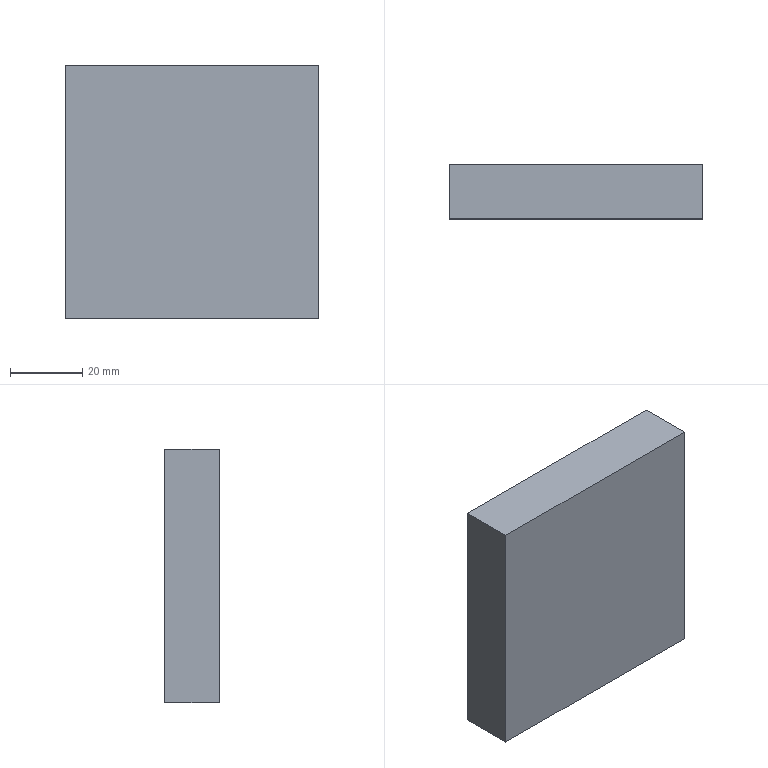Part | STEP file | Tube feed_id682_x_t | 1 solid | 6 faces | box 70 x 15 x 70 mm | volume 73500 mm3 | plane 6
STEP:
#1=CARTESIAN_POINT('',(0.,0.,0.));
#2=DIRECTION('',(0.,0.,1.));
#3=DIRECTION('',(1.,0.,0.));
#4=AXIS2_PLACEMENT_3D('',#1,#2,#3);
#5=CARTESIAN_POINT('',(141.,175.936,-50.15));
#6=VERTEX_POINT('',#5);
#7=CARTESIAN_POINT('',(141.,160.936,-50.15));
#8=VERTEX_POINT('',#7);
#9=CARTESIAN_POINT('',(141.,175.936,-50.15));
#10=DIRECTION('',(0.,-1.,0.));
#11=VECTOR('',#10,1.);
#12=LINE('',#9,#11);
#13=CARTESIAN_POINT('',(141.,175.936,19.85));
#14=DIRECTION('',(1.,0.,0.));
#15=DIRECTION('',(0.,0.,-1.));
#16=AXIS2_PLACEMENT_3D('',#13,#14,#15);
#17=PLANE('',#16);
#18=CARTESIAN_POINT('',(70.,0.));
#19=DIRECTION('',(0.,-1.));
#20=VECTOR('',#19,1.);
#21=LINE('',#18,#20);
#22=(GEOMETRIC_REPRESENTATION_CONTEXT(2)PARAMETRIC_REPRESENTATION_CONTEXT()REPRESENTATION_CONTEXT('',''));
#23=DEFINITIONAL_REPRESENTATION('',(#21),#22);
#24=PCURVE('',#17,#23);
#25=CARTESIAN_POINT('',(0.,0.,-50.15));
#26=DIRECTION('',(0.,0.,1.));
#27=DIRECTION('',(1.,0.,0.));
#28=AXIS2_PLACEMENT_3D('',#25,#26,#27);
#29=PLANE('',#28);
#30=CARTESIAN_POINT('',(141.,175.936));
#31=DIRECTION('',(0.,-1.));
#32=VECTOR('',#31,1.);
#33=LINE('',#30,#32);
#34=(GEOMETRIC_REPRESENTATION_CONTEXT(2)PARAMETRIC_REPRESENTATION_CONTEXT()REPRESENTATION_CONTEXT('',''));
#35=DEFINITIONAL_REPRESENTATION('',(#33),#34);
#36=PCURVE('',#29,#35);
#37=SURFACE_CURVE('',#12,(#24,#36),.PCURVE_S1.);
#38=EDGE_CURVE('',#6,#8,#37,.T.);
#39=ORIENTED_EDGE('',*,*,#38,.T.);
#40=CARTESIAN_POINT('',(141.,160.936,19.85));
#41=VERTEX_POINT('',#40);
#42=CARTESIAN_POINT('',(141.,160.936,19.85));
#43=DIRECTION('',(0.,0.,-1.));
#44=VECTOR('',#43,1.);
#45=LINE('',#42,#44);
#46=CARTESIAN_POINT('',(0.,-15.));
#47=DIRECTION('',(1.,0.));
#48=VECTOR('',#47,1.);
#49=LINE('',#46,#48);
#50=(GEOMETRIC_REPRESENTATION_CONTEXT(2)PARAMETRIC_REPRESENTATION_CONTEXT()REPRESENTATION_CONTEXT('',''));
#51=DEFINITIONAL_REPRESENTATION('',(#49),#50);
#52=PCURVE('',#17,#51);
#53=CARTESIAN_POINT('',(141.,160.936,19.85));
#54=DIRECTION('',(0.,1.,0.));
#55=DIRECTION('',(-1.,0.,0.));
#56=AXIS2_PLACEMENT_3D('',#53,#54,#55);
#57=PLANE('',#56);
#58=CARTESIAN_POINT('',(0.,0.));
#59=DIRECTION('',(0.,-1.));
#60=VECTOR('',#59,1.);
#61=LINE('',#58,#60);
#62=(GEOMETRIC_REPRESENTATION_CONTEXT(2)PARAMETRIC_REPRESENTATION_CONTEXT()REPRESENTATION_CONTEXT('',''));
#63=DEFINITIONAL_REPRESENTATION('',(#61),#62);
#64=PCURVE('',#57,#63);
#65=SURFACE_CURVE('',#45,(#52,#64),.PCURVE_S1.);
#66=EDGE_CURVE('',#41,#8,#65,.T.);
#67=ORIENTED_EDGE('',*,*,#66,.F.);
#68=CARTESIAN_POINT('',(141.,175.936,19.85));
#69=VERTEX_POINT('',#68);
#70=CARTESIAN_POINT('',(141.,175.936,19.85));
#71=DIRECTION('',(0.,-1.,0.));
#72=VECTOR('',#71,1.);
#73=LINE('',#70,#72);
#74=CARTESIAN_POINT('',(0.,0.));
#75=DIRECTION('',(0.,-1.));
#76=VECTOR('',#75,1.);
#77=LINE('',#74,#76);
#78=(GEOMETRIC_REPRESENTATION_CONTEXT(2)PARAMETRIC_REPRESENTATION_CONTEXT()REPRESENTATION_CONTEXT('',''));
#79=DEFINITIONAL_REPRESENTATION('',(#77),#78);
#80=PCURVE('',#17,#79);
#81=CARTESIAN_POINT('',(0.,0.,19.85));
#82=DIRECTION('',(0.,0.,1.));
#83=DIRECTION('',(1.,0.,0.));
#84=AXIS2_PLACEMENT_3D('',#81,#82,#83);
#85=PLANE('',#84);
#86=CARTESIAN_POINT('',(141.,175.936));
#87=DIRECTION('',(0.,-1.));
#88=VECTOR('',#87,1.);
#89=LINE('',#86,#88);
#90=(GEOMETRIC_REPRESENTATION_CONTEXT(2)PARAMETRIC_REPRESENTATION_CONTEXT()REPRESENTATION_CONTEXT('',''));
#91=DEFINITIONAL_REPRESENTATION('',(#89),#90);
#92=PCURVE('',#85,#91);
#93=SURFACE_CURVE('',#73,(#80,#92),.PCURVE_S1.);
#94=EDGE_CURVE('',#69,#41,#93,.T.);
#95=ORIENTED_EDGE('',*,*,#94,.F.);
#96=CARTESIAN_POINT('',(141.,175.936,19.85));
#97=DIRECTION('',(0.,0.,-1.));
#98=VECTOR('',#97,1.);
#99=LINE('',#96,#98);
#100=CARTESIAN_POINT('',(0.,0.));
#101=DIRECTION('',(1.,0.));
#102=VECTOR('',#101,1.);
#103=LINE('',#100,#102);
#104=(GEOMETRIC_REPRESENTATION_CONTEXT(2)PARAMETRIC_REPRESENTATION_CONTEXT()REPRESENTATION_CONTEXT('',''));
#105=DEFINITIONAL_REPRESENTATION('',(#103),#104);
#106=PCURVE('',#17,#105);
#107=CARTESIAN_POINT('',(211.,175.936,19.85));
#108=DIRECTION('',(0.,-1.,0.));
#109=DIRECTION('',(0.,0.,-1.));
#110=AXIS2_PLACEMENT_3D('',#107,#108,#109);
#111=PLANE('',#110);
#112=CARTESIAN_POINT('',(0.,-70.));
#113=DIRECTION('',(1.,0.));
#114=VECTOR('',#113,1.);
#115=LINE('',#112,#114);
#116=(GEOMETRIC_REPRESENTATION_CONTEXT(2)PARAMETRIC_REPRESENTATION_CONTEXT()REPRESENTATION_CONTEXT('',''));
#117=DEFINITIONAL_REPRESENTATION('',(#115),#116);
#118=PCURVE('',#111,#117);
#119=SURFACE_CURVE('',#99,(#106,#118),.PCURVE_S1.);
#120=EDGE_CURVE('',#69,#6,#119,.T.);
#121=ORIENTED_EDGE('',*,*,#120,.T.);
#122=EDGE_LOOP('',(#39,#67,#95,#121));
#123=FACE_BOUND('',#122,.T.);
#124=ADVANCED_FACE('',(#123),#17,.F.);
#125=CARTESIAN_POINT('',(211.,160.936,-50.15));
#126=VERTEX_POINT('',#125);
#127=CARTESIAN_POINT('',(141.,160.936,-50.15));
#128=DIRECTION('',(1.,0.,0.));
#129=VECTOR('',#128,1.);
#130=LINE('',#127,#129);
#131=CARTESIAN_POINT('',(0.,-70.));
#132=DIRECTION('',(-1.,0.));
#133=VECTOR('',#132,1.);
#134=LINE('',#131,#133);
#135=(GEOMETRIC_REPRESENTATION_CONTEXT(2)PARAMETRIC_REPRESENTATION_CONTEXT()REPRESENTATION_CONTEXT('',''));
#136=DEFINITIONAL_REPRESENTATION('',(#134),#135);
#137=PCURVE('',#57,#136);
#138=CARTESIAN_POINT('',(141.,160.936));
#139=DIRECTION('',(1.,0.));
#140=VECTOR('',#139,1.);
#141=LINE('',#138,#140);
#142=(GEOMETRIC_REPRESENTATION_CONTEXT(2)PARAMETRIC_REPRESENTATION_CONTEXT()REPRESENTATION_CONTEXT('',''));
#143=DEFINITIONAL_REPRESENTATION('',(#141),#142);
#144=PCURVE('',#29,#143);
#145=SURFACE_CURVE('',#130,(#137,#144),.PCURVE_S1.);
#146=EDGE_CURVE('',#8,#126,#145,.T.);
#147=ORIENTED_EDGE('',*,*,#146,.T.);
#148=CARTESIAN_POINT('',(211.,160.936,19.85));
#149=VERTEX_POINT('',#148);
#150=CARTESIAN_POINT('',(211.,160.936,19.85));
#151=DIRECTION('',(0.,0.,-1.));
#152=VECTOR('',#151,1.);
#153=LINE('',#150,#152);
#154=CARTESIAN_POINT('',(-70.,0.));
#155=DIRECTION('',(0.,-1.));
#156=VECTOR('',#155,1.);
#157=LINE('',#154,#156);
#158=(GEOMETRIC_REPRESENTATION_CONTEXT(2)PARAMETRIC_REPRESENTATION_CONTEXT()REPRESENTATION_CONTEXT('',''));
#159=DEFINITIONAL_REPRESENTATION('',(#157),#158);
#160=PCURVE('',#57,#159);
#161=CARTESIAN_POINT('',(211.,160.936,19.85));
#162=DIRECTION('',(-1.,0.,0.));
#163=DIRECTION('',(0.,0.,1.));
#164=AXIS2_PLACEMENT_3D('',#161,#162,#163);
#165=PLANE('',#164);
#166=CARTESIAN_POINT('',(0.,0.));
#167=DIRECTION('',(-1.,0.));
#168=VECTOR('',#167,1.);
#169=LINE('',#166,#168);
#170=(GEOMETRIC_REPRESENTATION_CONTEXT(2)PARAMETRIC_REPRESENTATION_CONTEXT()REPRESENTATION_CONTEXT('',''));
#171=DEFINITIONAL_REPRESENTATION('',(#169),#170);
#172=PCURVE('',#165,#171);
#173=SURFACE_CURVE('',#153,(#160,#172),.PCURVE_S1.);
#174=EDGE_CURVE('',#149,#126,#173,.T.);
#175=ORIENTED_EDGE('',*,*,#174,.F.);
#176=CARTESIAN_POINT('',(141.,160.936,19.85));
#177=DIRECTION('',(1.,0.,0.));
#178=VECTOR('',#177,1.);
#179=LINE('',#176,#178);
#180=CARTESIAN_POINT('',(0.,0.));
#181=DIRECTION('',(-1.,0.));
#182=VECTOR('',#181,1.);
#183=LINE('',#180,#182);
#184=(GEOMETRIC_REPRESENTATION_CONTEXT(2)PARAMETRIC_REPRESENTATION_CONTEXT()REPRESENTATION_CONTEXT('',''));
#185=DEFINITIONAL_REPRESENTATION('',(#183),#184);
#186=PCURVE('',#57,#185);
#187=CARTESIAN_POINT('',(141.,160.936));
#188=DIRECTION('',(1.,0.));
#189=VECTOR('',#188,1.);
#190=LINE('',#187,#189);
#191=(GEOMETRIC_REPRESENTATION_CONTEXT(2)PARAMETRIC_REPRESENTATION_CONTEXT()REPRESENTATION_CONTEXT('',''));
#192=DEFINITIONAL_REPRESENTATION('',(#190),#191);
#193=PCURVE('',#85,#192);
#194=SURFACE_CURVE('',#179,(#186,#193),.PCURVE_S1.);
#195=EDGE_CURVE('',#41,#149,#194,.T.);
#196=ORIENTED_EDGE('',*,*,#195,.F.);
#197=ORIENTED_EDGE('',*,*,#66,.T.);
#198=EDGE_LOOP('',(#147,#175,#196,#197));
#199=FACE_BOUND('',#198,.T.);
#200=ADVANCED_FACE('',(#199),#57,.F.);
#201=CARTESIAN_POINT('',(211.,175.936,-50.15));
#202=VERTEX_POINT('',#201);
#203=CARTESIAN_POINT('',(211.,160.936,-50.15));
#204=DIRECTION('',(0.,1.,0.));
#205=VECTOR('',#204,1.);
#206=LINE('',#203,#205);
#207=CARTESIAN_POINT('',(-70.,0.));
#208=DIRECTION('',(0.,1.));
#209=VECTOR('',#208,1.);
#210=LINE('',#207,#209);
#211=(GEOMETRIC_REPRESENTATION_CONTEXT(2)PARAMETRIC_REPRESENTATION_CONTEXT()REPRESENTATION_CONTEXT('',''));
#212=DEFINITIONAL_REPRESENTATION('',(#210),#211);
#213=PCURVE('',#165,#212);
#214=CARTESIAN_POINT('',(211.,160.936));
#215=DIRECTION('',(0.,1.));
#216=VECTOR('',#215,1.);
#217=LINE('',#214,#216);
#218=(GEOMETRIC_REPRESENTATION_CONTEXT(2)PARAMETRIC_REPRESENTATION_CONTEXT()REPRESENTATION_CONTEXT('',''));
#219=DEFINITIONAL_REPRESENTATION('',(#217),#218);
#220=PCURVE('',#29,#219);
#221=SURFACE_CURVE('',#206,(#213,#220),.PCURVE_S1.);
#222=EDGE_CURVE('',#126,#202,#221,.T.);
#223=ORIENTED_EDGE('',*,*,#222,.T.);
#224=CARTESIAN_POINT('',(211.,175.936,19.85));
#225=VERTEX_POINT('',#224);
#226=CARTESIAN_POINT('',(211.,175.936,19.85));
#227=DIRECTION('',(0.,0.,-1.));
#228=VECTOR('',#227,1.);
#229=LINE('',#226,#228);
#230=CARTESIAN_POINT('',(0.,15.));
#231=DIRECTION('',(-1.,0.));
#232=VECTOR('',#231,1.);
#233=LINE('',#230,#232);
#234=(GEOMETRIC_REPRESENTATION_CONTEXT(2)PARAMETRIC_REPRESENTATION_CONTEXT()REPRESENTATION_CONTEXT('',''));
#235=DEFINITIONAL_REPRESENTATION('',(#233),#234);
#236=PCURVE('',#165,#235);
#237=CARTESIAN_POINT('',(0.,0.));
#238=DIRECTION('',(1.,0.));
#239=VECTOR('',#238,1.);
#240=LINE('',#237,#239);
#241=(GEOMETRIC_REPRESENTATION_CONTEXT(2)PARAMETRIC_REPRESENTATION_CONTEXT()REPRESENTATION_CONTEXT('',''));
#242=DEFINITIONAL_REPRESENTATION('',(#240),#241);
#243=PCURVE('',#111,#242);
#244=SURFACE_CURVE('',#229,(#236,#243),.PCURVE_S1.);
#245=EDGE_CURVE('',#225,#202,#244,.T.);
#246=ORIENTED_EDGE('',*,*,#245,.F.);
#247=CARTESIAN_POINT('',(211.,160.936,19.85));
#248=DIRECTION('',(0.,1.,0.));
#249=VECTOR('',#248,1.);
#250=LINE('',#247,#249);
#251=CARTESIAN_POINT('',(0.,0.));
#252=DIRECTION('',(0.,1.));
#253=VECTOR('',#252,1.);
#254=LINE('',#251,#253);
#255=(GEOMETRIC_REPRESENTATION_CONTEXT(2)PARAMETRIC_REPRESENTATION_CONTEXT()REPRESENTATION_CONTEXT('',''));
#256=DEFINITIONAL_REPRESENTATION('',(#254),#255);
#257=PCURVE('',#165,#256);
#258=CARTESIAN_POINT('',(211.,160.936));
#259=DIRECTION('',(0.,1.));
#260=VECTOR('',#259,1.);
#261=LINE('',#258,#260);
#262=(GEOMETRIC_REPRESENTATION_CONTEXT(2)PARAMETRIC_REPRESENTATION_CONTEXT()REPRESENTATION_CONTEXT('',''));
#263=DEFINITIONAL_REPRESENTATION('',(#261),#262);
#264=PCURVE('',#85,#263);
#265=SURFACE_CURVE('',#250,(#257,#264),.PCURVE_S1.);
#266=EDGE_CURVE('',#149,#225,#265,.T.);
#267=ORIENTED_EDGE('',*,*,#266,.F.);
#268=ORIENTED_EDGE('',*,*,#174,.T.);
#269=EDGE_LOOP('',(#223,#246,#267,#268));
#270=FACE_BOUND('',#269,.T.);
#271=ADVANCED_FACE('',(#270),#165,.F.);
#272=CARTESIAN_POINT('',(211.,175.936,-50.15));
#273=DIRECTION('',(-1.,0.,0.));
#274=VECTOR('',#273,1.);
#275=LINE('',#272,#274);
#276=CARTESIAN_POINT('',(70.,0.));
#277=DIRECTION('',(0.,-1.));
#278=VECTOR('',#277,1.);
#279=LINE('',#276,#278);
#280=(GEOMETRIC_REPRESENTATION_CONTEXT(2)PARAMETRIC_REPRESENTATION_CONTEXT()REPRESENTATION_CONTEXT('',''));
#281=DEFINITIONAL_REPRESENTATION('',(#279),#280);
#282=PCURVE('',#111,#281);
#283=CARTESIAN_POINT('',(211.,175.936));
#284=DIRECTION('',(-1.,0.));
#285=VECTOR('',#284,1.);
#286=LINE('',#283,#285);
#287=(GEOMETRIC_REPRESENTATION_CONTEXT(2)PARAMETRIC_REPRESENTATION_CONTEXT()REPRESENTATION_CONTEXT('',''));
#288=DEFINITIONAL_REPRESENTATION('',(#286),#287);
#289=PCURVE('',#29,#288);
#290=SURFACE_CURVE('',#275,(#282,#289),.PCURVE_S1.);
#291=EDGE_CURVE('',#202,#6,#290,.T.);
#292=ORIENTED_EDGE('',*,*,#291,.T.);
#293=ORIENTED_EDGE('',*,*,#120,.F.);
#294=CARTESIAN_POINT('',(211.,175.936,19.85));
#295=DIRECTION('',(-1.,0.,0.));
#296=VECTOR('',#295,1.);
#297=LINE('',#294,#296);
#298=CARTESIAN_POINT('',(0.,0.));
#299=DIRECTION('',(0.,-1.));
#300=VECTOR('',#299,1.);
#301=LINE('',#298,#300);
#302=(GEOMETRIC_REPRESENTATION_CONTEXT(2)PARAMETRIC_REPRESENTATION_CONTEXT()REPRESENTATION_CONTEXT('',''));
#303=DEFINITIONAL_REPRESENTATION('',(#301),#302);
#304=PCURVE('',#111,#303);
#305=CARTESIAN_POINT('',(211.,175.936));
#306=DIRECTION('',(-1.,0.));
#307=VECTOR('',#306,1.);
#308=LINE('',#305,#307);
#309=(GEOMETRIC_REPRESENTATION_CONTEXT(2)PARAMETRIC_REPRESENTATION_CONTEXT()REPRESENTATION_CONTEXT('',''));
#310=DEFINITIONAL_REPRESENTATION('',(#308),#309);
#311=PCURVE('',#85,#310);
#312=SURFACE_CURVE('',#297,(#304,#311),.PCURVE_S1.);
#313=EDGE_CURVE('',#225,#69,#312,.T.);
#314=ORIENTED_EDGE('',*,*,#313,.F.);
#315=ORIENTED_EDGE('',*,*,#245,.T.);
#316=EDGE_LOOP('',(#292,#293,#314,#315));
#317=FACE_BOUND('',#316,.T.);
#318=ADVANCED_FACE('',(#317),#111,.F.);
#319=ORIENTED_EDGE('',*,*,#94,.T.);
#320=ORIENTED_EDGE('',*,*,#195,.T.);
#321=ORIENTED_EDGE('',*,*,#266,.T.);
#322=ORIENTED_EDGE('',*,*,#313,.T.);
#323=EDGE_LOOP('',(#319,#320,#321,#322));
#324=FACE_BOUND('',#323,.T.);
#325=ADVANCED_FACE('',(#324),#85,.T.);
#326=ORIENTED_EDGE('',*,*,#38,.F.);
#327=ORIENTED_EDGE('',*,*,#291,.F.);
#328=ORIENTED_EDGE('',*,*,#222,.F.);
#329=ORIENTED_EDGE('',*,*,#146,.F.);
#330=EDGE_LOOP('',(#326,#327,#328,#329));
#331=FACE_BOUND('',#330,.T.);
#332=ADVANCED_FACE('',(#331),#29,.F.);
#333=CLOSED_SHELL('',(#124,#200,#271,#318,#325,#332));
#334=MANIFOLD_SOLID_BREP('',#333);
#335=(LENGTH_UNIT()NAMED_UNIT(*)SI_UNIT(.MILLI.,.METRE.));
#336=UNCERTAINTY_MEASURE_WITH_UNIT(LENGTH_MEASURE(0.0000001),#335,'','');
#337=(NAMED_UNIT(*)PLANE_ANGLE_UNIT()SI_UNIT($,.RADIAN.));
#338=(NAMED_UNIT(*)SI_UNIT($,.STERADIAN.)SOLID_ANGLE_UNIT());
#339=(GEOMETRIC_REPRESENTATION_CONTEXT(3)GLOBAL_UNCERTAINTY_ASSIGNED_CONTEXT((#336))GLOBAL_UNIT_ASSIGNED_CONTEXT((#335,#337,#338))REPRESENTATION_CONTEXT('',''));
#340=ADVANCED_BREP_SHAPE_REPRESENTATION('',(#4,#334),#339);